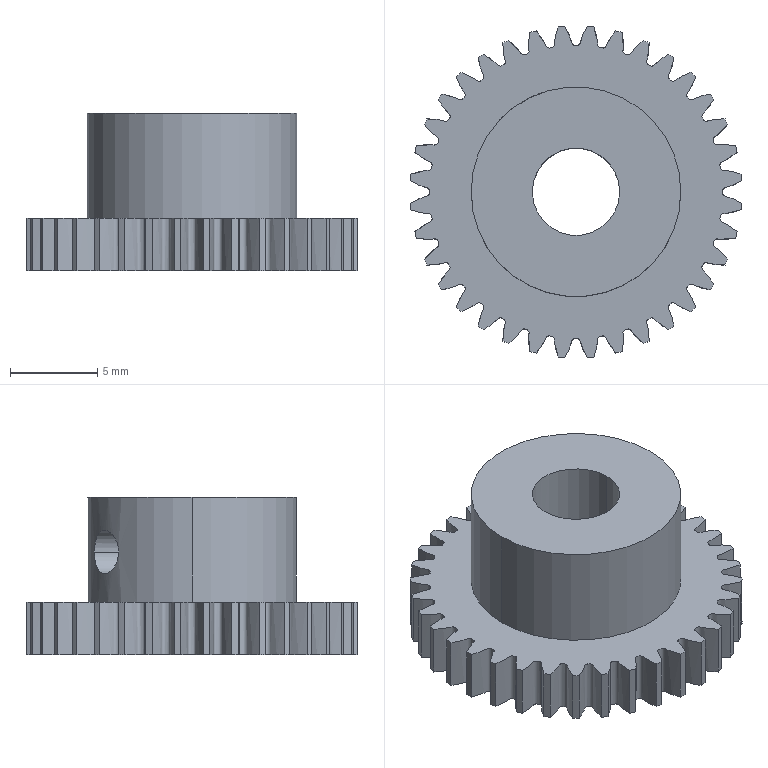Part | SolidWorks | features ICE 3, 3DProfileFeature 1, CirPattern 1, HoleWzd 1, RefAxis 1, Revolution 1 | 1 solid | 81 faces | box 18.957 x 18.957 x 9 mm | volume 1231 mm3 | cylinder 42 | spline 36 | plane 3 | commonest cylinder face diameters 19 x36 2.5 x2 5 x2 12 x2